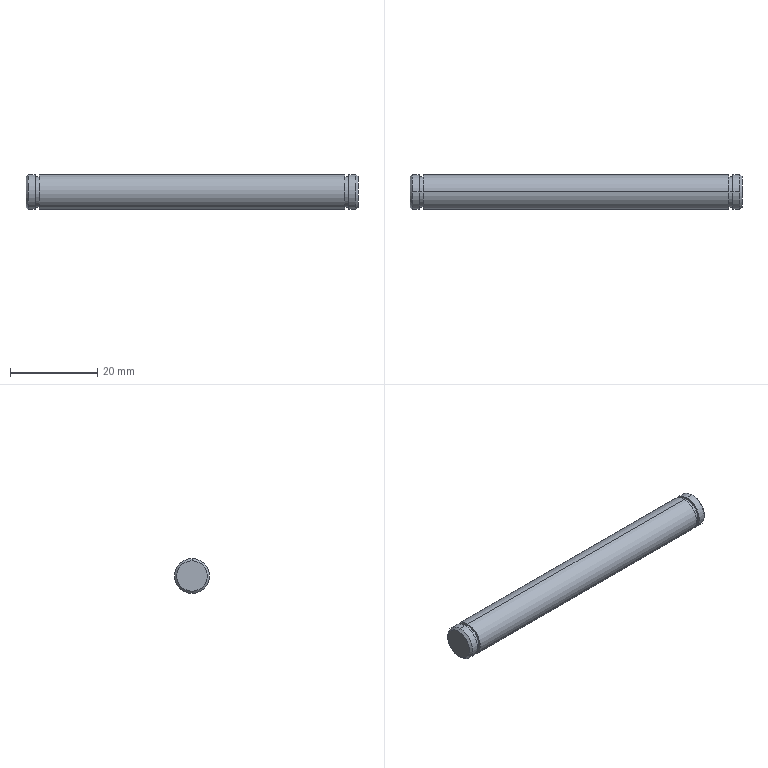Part | NX | features BREP 1 | 1 solid | 20 faces | box 76 x 8 x 8 mm | volume 3793 mm3 | cylinder 10 | plane 6 | cone 4 | commonest cylinder face diameters 8 x6 7 x4
STEP:
#1=CARTESIAN_POINT('',(76.,0.,3.5));
#2=VERTEX_POINT('',#1);
#3=CARTESIAN_POINT('',(76.,0.,-3.5));
#4=VERTEX_POINT('',#3);
#5=CARTESIAN_POINT('',(76.,0.,0.));
#6=DIRECTION('',(-1.,0.,0.));
#7=DIRECTION('',(0.,0.,1.));
#8=AXIS2_PLACEMENT_3D('',#5,#6,#7);
#9=CIRCLE('',#8,3.5);
#10=EDGE_CURVE('',#2,#4,#9,.T.);
#11=ORIENTED_EDGE('',*,*,#10,.T.);
#12=CARTESIAN_POINT('',(75.5,0.,-4.));
#13=VERTEX_POINT('',#12);
#14=CARTESIAN_POINT('',(76.,0.,-3.5));
#15=DIRECTION('',(-0.7071,0.,-0.7071));
#16=VECTOR('',#15,1000.);
#17=LINE('',#14,#16);
#18=EDGE_CURVE('',#13,#4,#17,.F.);
#19=ORIENTED_EDGE('',*,*,#18,.F.);
#20=CARTESIAN_POINT('',(75.5,0.,4.));
#21=VERTEX_POINT('',#20);
#22=CARTESIAN_POINT('',(75.5,0.,0.));
#23=DIRECTION('',(-1.,0.,0.));
#24=DIRECTION('',(0.,0.,1.));
#25=AXIS2_PLACEMENT_3D('',#22,#23,#24);
#26=CIRCLE('',#25,4.);
#27=EDGE_CURVE('',#21,#13,#26,.T.);
#28=ORIENTED_EDGE('',*,*,#27,.F.);
#29=CARTESIAN_POINT('',(76.,0.,3.5));
#30=DIRECTION('',(-0.7071,0.,0.7071));
#31=VECTOR('',#30,1000.);
#32=LINE('',#29,#31);
#33=EDGE_CURVE('',#21,#2,#32,.F.);
#34=ORIENTED_EDGE('',*,*,#33,.T.);
#35=EDGE_LOOP('',(#11,#19,#28,#34));
#36=FACE_BOUND('',#35,.T.);
#37=CARTESIAN_POINT('',(76.,0.,0.));
#38=DIRECTION('',(-1.,0.,0.));
#39=DIRECTION('',(0.,0.,1.));
#40=AXIS2_PLACEMENT_3D('',#37,#38,#39);
#41=CONICAL_SURFACE('',#40,3.5,0.7854);
#42=ADVANCED_FACE('',(#36),#41,.T.);
#43=ORIENTED_EDGE('',*,*,#27,.T.);
#44=CARTESIAN_POINT('',(73.9,0.,-4.));
#45=VERTEX_POINT('',#44);
#46=CARTESIAN_POINT('',(76.,0.,-4.));
#47=DIRECTION('',(-1.,0.,0.));
#48=VECTOR('',#47,1000.);
#49=LINE('',#46,#48);
#50=EDGE_CURVE('',#45,#13,#49,.F.);
#51=ORIENTED_EDGE('',*,*,#50,.F.);
#52=CARTESIAN_POINT('',(73.9,0.,4.));
#53=VERTEX_POINT('',#52);
#54=CARTESIAN_POINT('',(73.9,0.,0.));
#55=DIRECTION('',(-1.,0.,0.));
#56=DIRECTION('',(0.,0.,1.));
#57=AXIS2_PLACEMENT_3D('',#54,#55,#56);
#58=CIRCLE('',#57,4.);
#59=EDGE_CURVE('',#53,#45,#58,.T.);
#60=ORIENTED_EDGE('',*,*,#59,.F.);
#61=CARTESIAN_POINT('',(76.,0.,4.));
#62=DIRECTION('',(-1.,0.,0.));
#63=VECTOR('',#62,1000.);
#64=LINE('',#61,#63);
#65=EDGE_CURVE('',#53,#21,#64,.F.);
#66=ORIENTED_EDGE('',*,*,#65,.T.);
#67=EDGE_LOOP('',(#43,#51,#60,#66));
#68=FACE_BOUND('',#67,.T.);
#69=CARTESIAN_POINT('',(76.,0.,0.));
#70=DIRECTION('',(-1.,0.,0.));
#71=DIRECTION('',(0.,0.,1.));
#72=AXIS2_PLACEMENT_3D('',#69,#70,#71);
#73=CYLINDRICAL_SURFACE('',#72,4.);
#74=ADVANCED_FACE('',(#68),#73,.T.);
#75=CARTESIAN_POINT('',(73.9,0.,3.5));
#76=VERTEX_POINT('',#75);
#77=CARTESIAN_POINT('',(73.9,0.,-3.5));
#78=VERTEX_POINT('',#77);
#79=CARTESIAN_POINT('',(73.9,0.,0.));
#80=DIRECTION('',(-1.,0.,0.));
#81=DIRECTION('',(0.,0.,1.));
#82=AXIS2_PLACEMENT_3D('',#79,#80,#81);
#83=CIRCLE('',#82,3.5);
#84=EDGE_CURVE('',#76,#78,#83,.T.);
#85=ORIENTED_EDGE('',*,*,#84,.T.);
#86=CARTESIAN_POINT('',(73.,0.,-3.5));
#87=VERTEX_POINT('',#86);
#88=CARTESIAN_POINT('',(76.,0.,-3.5));
#89=DIRECTION('',(-1.,0.,0.));
#90=VECTOR('',#89,1000.);
#91=LINE('',#88,#90);
#92=EDGE_CURVE('',#87,#78,#91,.F.);
#93=ORIENTED_EDGE('',*,*,#92,.F.);
#94=CARTESIAN_POINT('',(73.,0.,3.5));
#95=VERTEX_POINT('',#94);
#96=CARTESIAN_POINT('',(73.,0.,0.));
#97=DIRECTION('',(-1.,0.,0.));
#98=DIRECTION('',(0.,0.,1.));
#99=AXIS2_PLACEMENT_3D('',#96,#97,#98);
#100=CIRCLE('',#99,3.5);
#101=EDGE_CURVE('',#95,#87,#100,.T.);
#102=ORIENTED_EDGE('',*,*,#101,.F.);
#103=CARTESIAN_POINT('',(76.,0.,3.5));
#104=DIRECTION('',(-1.,0.,0.));
#105=VECTOR('',#104,1000.);
#106=LINE('',#103,#105);
#107=EDGE_CURVE('',#95,#76,#106,.F.);
#108=ORIENTED_EDGE('',*,*,#107,.T.);
#109=EDGE_LOOP('',(#85,#93,#102,#108));
#110=FACE_BOUND('',#109,.T.);
#111=CARTESIAN_POINT('',(76.,0.,0.));
#112=DIRECTION('',(-1.,0.,0.));
#113=DIRECTION('',(0.,0.,1.));
#114=AXIS2_PLACEMENT_3D('',#111,#112,#113);
#115=CYLINDRICAL_SURFACE('',#114,3.5);
#116=ADVANCED_FACE('',(#110),#115,.T.);
#117=CARTESIAN_POINT('',(73.,0.,4.));
#118=VERTEX_POINT('',#117);
#119=CARTESIAN_POINT('',(73.,0.,-4.));
#120=VERTEX_POINT('',#119);
#121=CARTESIAN_POINT('',(73.,0.,0.));
#122=DIRECTION('',(-1.,0.,0.));
#123=DIRECTION('',(0.,0.,1.));
#124=AXIS2_PLACEMENT_3D('',#121,#122,#123);
#125=CIRCLE('',#124,4.);
#126=EDGE_CURVE('',#118,#120,#125,.T.);
#127=ORIENTED_EDGE('',*,*,#126,.T.);
#128=CARTESIAN_POINT('',(3.,0.,-4.));
#129=VERTEX_POINT('',#128);
#130=CARTESIAN_POINT('',(76.,0.,-4.));
#131=DIRECTION('',(-1.,0.,0.));
#132=VECTOR('',#131,1000.);
#133=LINE('',#130,#132);
#134=EDGE_CURVE('',#129,#120,#133,.F.);
#135=ORIENTED_EDGE('',*,*,#134,.F.);
#136=CARTESIAN_POINT('',(3.,0.,4.));
#137=VERTEX_POINT('',#136);
#138=CARTESIAN_POINT('',(3.,0.,0.));
#139=DIRECTION('',(-1.,0.,0.));
#140=DIRECTION('',(0.,0.,1.));
#141=AXIS2_PLACEMENT_3D('',#138,#139,#140);
#142=CIRCLE('',#141,4.);
#143=EDGE_CURVE('',#137,#129,#142,.T.);
#144=ORIENTED_EDGE('',*,*,#143,.F.);
#145=CARTESIAN_POINT('',(76.,0.,4.));
#146=DIRECTION('',(-1.,0.,0.));
#147=VECTOR('',#146,1000.);
#148=LINE('',#145,#147);
#149=EDGE_CURVE('',#137,#118,#148,.F.);
#150=ORIENTED_EDGE('',*,*,#149,.T.);
#151=EDGE_LOOP('',(#127,#135,#144,#150));
#152=FACE_BOUND('',#151,.T.);
#153=CARTESIAN_POINT('',(76.,0.,0.));
#154=DIRECTION('',(-1.,0.,0.));
#155=DIRECTION('',(0.,0.,1.));
#156=AXIS2_PLACEMENT_3D('',#153,#154,#155);
#157=CYLINDRICAL_SURFACE('',#156,4.);
#158=ADVANCED_FACE('',(#152),#157,.T.);
#159=CARTESIAN_POINT('',(3.,0.,3.5));
#160=VERTEX_POINT('',#159);
#161=CARTESIAN_POINT('',(3.,0.,-3.5));
#162=VERTEX_POINT('',#161);
#163=CARTESIAN_POINT('',(3.,0.,0.));
#164=DIRECTION('',(-1.,0.,0.));
#165=DIRECTION('',(0.,0.,1.));
#166=AXIS2_PLACEMENT_3D('',#163,#164,#165);
#167=CIRCLE('',#166,3.5);
#168=EDGE_CURVE('',#160,#162,#167,.T.);
#169=ORIENTED_EDGE('',*,*,#168,.T.);
#170=CARTESIAN_POINT('',(2.1,0.,-3.5));
#171=VERTEX_POINT('',#170);
#172=CARTESIAN_POINT('',(76.,0.,-3.5));
#173=DIRECTION('',(-1.,0.,0.));
#174=VECTOR('',#173,1000.);
#175=LINE('',#172,#174);
#176=EDGE_CURVE('',#171,#162,#175,.F.);
#177=ORIENTED_EDGE('',*,*,#176,.F.);
#178=CARTESIAN_POINT('',(2.1,0.,3.5));
#179=VERTEX_POINT('',#178);
#180=CARTESIAN_POINT('',(2.1,0.,0.));
#181=DIRECTION('',(-1.,0.,0.));
#182=DIRECTION('',(0.,0.,1.));
#183=AXIS2_PLACEMENT_3D('',#180,#181,#182);
#184=CIRCLE('',#183,3.5);
#185=EDGE_CURVE('',#179,#171,#184,.T.);
#186=ORIENTED_EDGE('',*,*,#185,.F.);
#187=CARTESIAN_POINT('',(76.,0.,3.5));
#188=DIRECTION('',(-1.,0.,0.));
#189=VECTOR('',#188,1000.);
#190=LINE('',#187,#189);
#191=EDGE_CURVE('',#179,#160,#190,.F.);
#192=ORIENTED_EDGE('',*,*,#191,.T.);
#193=EDGE_LOOP('',(#169,#177,#186,#192));
#194=FACE_BOUND('',#193,.T.);
#195=CARTESIAN_POINT('',(76.,0.,0.));
#196=DIRECTION('',(-1.,0.,0.));
#197=DIRECTION('',(0.,0.,1.));
#198=AXIS2_PLACEMENT_3D('',#195,#196,#197);
#199=CYLINDRICAL_SURFACE('',#198,3.5);
#200=ADVANCED_FACE('',(#194),#199,.T.);
#201=CARTESIAN_POINT('',(2.1,0.,4.));
#202=VERTEX_POINT('',#201);
#203=CARTESIAN_POINT('',(2.1,0.,-4.));
#204=VERTEX_POINT('',#203);
#205=CARTESIAN_POINT('',(2.1,0.,0.));
#206=DIRECTION('',(-1.,0.,0.));
#207=DIRECTION('',(0.,0.,1.));
#208=AXIS2_PLACEMENT_3D('',#205,#206,#207);
#209=CIRCLE('',#208,4.);
#210=EDGE_CURVE('',#202,#204,#209,.T.);
#211=ORIENTED_EDGE('',*,*,#210,.T.);
#212=CARTESIAN_POINT('',(0.5,0.,-4.));
#213=VERTEX_POINT('',#212);
#214=CARTESIAN_POINT('',(76.,0.,-4.));
#215=DIRECTION('',(-1.,0.,0.));
#216=VECTOR('',#215,1000.);
#217=LINE('',#214,#216);
#218=EDGE_CURVE('',#213,#204,#217,.F.);
#219=ORIENTED_EDGE('',*,*,#218,.F.);
#220=CARTESIAN_POINT('',(0.5,0.,4.));
#221=VERTEX_POINT('',#220);
#222=CARTESIAN_POINT('',(0.5,0.,0.));
#223=DIRECTION('',(-1.,0.,0.));
#224=DIRECTION('',(0.,0.,1.));
#225=AXIS2_PLACEMENT_3D('',#222,#223,#224);
#226=CIRCLE('',#225,4.);
#227=EDGE_CURVE('',#221,#213,#226,.T.);
#228=ORIENTED_EDGE('',*,*,#227,.F.);
#229=CARTESIAN_POINT('',(76.,0.,4.));
#230=DIRECTION('',(-1.,0.,0.));
#231=VECTOR('',#230,1000.);
#232=LINE('',#229,#231);
#233=EDGE_CURVE('',#221,#202,#232,.F.);
#234=ORIENTED_EDGE('',*,*,#233,.T.);
#235=EDGE_LOOP('',(#211,#219,#228,#234));
#236=FACE_BOUND('',#235,.T.);
#237=CARTESIAN_POINT('',(76.,0.,0.));
#238=DIRECTION('',(-1.,0.,0.));
#239=DIRECTION('',(0.,0.,1.));
#240=AXIS2_PLACEMENT_3D('',#237,#238,#239);
#241=CYLINDRICAL_SURFACE('',#240,4.);
#242=ADVANCED_FACE('',(#236),#241,.T.);
#243=CARTESIAN_POINT('',(0.,0.,3.5));
#244=VERTEX_POINT('',#243);
#245=CARTESIAN_POINT('',(0.,0.,-3.5));
#246=VERTEX_POINT('',#245);
#247=CARTESIAN_POINT('',(0.,0.,0.));
#248=DIRECTION('',(-1.,0.,0.));
#249=DIRECTION('',(0.,0.,1.));
#250=AXIS2_PLACEMENT_3D('',#247,#248,#249);
#251=CIRCLE('',#250,3.5);
#252=EDGE_CURVE('',#244,#246,#251,.T.);
#253=ORIENTED_EDGE('',*,*,#252,.F.);
#254=CARTESIAN_POINT('',(0.5,0.,4.));
#255=DIRECTION('',(0.7071,0.,0.7071));
#256=VECTOR('',#255,1000.);
#257=LINE('',#254,#256);
#258=EDGE_CURVE('',#244,#221,#257,.T.);
#259=ORIENTED_EDGE('',*,*,#258,.T.);
#260=ORIENTED_EDGE('',*,*,#227,.T.);
#261=CARTESIAN_POINT('',(0.5,0.,-4.));
#262=DIRECTION('',(0.7071,0.,-0.7071));
#263=VECTOR('',#262,1000.);
#264=LINE('',#261,#263);
#265=EDGE_CURVE('',#246,#213,#264,.T.);
#266=ORIENTED_EDGE('',*,*,#265,.F.);
#267=EDGE_LOOP('',(#253,#259,#260,#266));
#268=FACE_BOUND('',#267,.T.);
#269=CARTESIAN_POINT('',(0.5,0.,0.));
#270=DIRECTION('',(1.,0.,0.));
#271=DIRECTION('',(0.,0.,-1.));
#272=AXIS2_PLACEMENT_3D('',#269,#270,#271);
#273=CONICAL_SURFACE('',#272,4.,0.7854);
#274=ADVANCED_FACE('',(#268),#273,.T.);
#275=CARTESIAN_POINT('',(0.,0.,0.));
#276=DIRECTION('',(-1.,0.,0.));
#277=DIRECTION('',(0.,0.,1.));
#278=AXIS2_PLACEMENT_3D('',#275,#276,#277);
#279=CIRCLE('',#278,3.5);
#280=EDGE_CURVE('',#246,#244,#279,.T.);
#281=ORIENTED_EDGE('',*,*,#280,.T.);
#282=ORIENTED_EDGE('',*,*,#252,.T.);
#283=EDGE_LOOP('',(#281,#282));
#284=FACE_BOUND('',#283,.T.);
#285=CARTESIAN_POINT('',(0.,0.,0.));
#286=DIRECTION('',(1.,0.,0.));
#287=DIRECTION('',(0.,1.,0.));
#288=AXIS2_PLACEMENT_3D('',#285,#286,#287);
#289=PLANE('',#288);
#290=ADVANCED_FACE('',(#284),#289,.F.);
#291=ORIENTED_EDGE('',*,*,#258,.F.);
#292=ORIENTED_EDGE('',*,*,#280,.F.);
#293=ORIENTED_EDGE('',*,*,#265,.T.);
#294=CARTESIAN_POINT('',(0.5,0.,0.));
#295=DIRECTION('',(-1.,0.,0.));
#296=DIRECTION('',(0.,0.,1.));
#297=AXIS2_PLACEMENT_3D('',#294,#295,#296);
#298=CIRCLE('',#297,4.);
#299=EDGE_CURVE('',#213,#221,#298,.T.);
#300=ORIENTED_EDGE('',*,*,#299,.T.);
#301=EDGE_LOOP('',(#291,#292,#293,#300));
#302=FACE_BOUND('',#301,.T.);
#303=CARTESIAN_POINT('',(0.5,0.,0.));
#304=DIRECTION('',(1.,0.,0.));
#305=DIRECTION('',(0.,0.,-1.));
#306=AXIS2_PLACEMENT_3D('',#303,#304,#305);
#307=CONICAL_SURFACE('',#306,4.,0.7854);
#308=ADVANCED_FACE('',(#302),#307,.T.);
#309=ORIENTED_EDGE('',*,*,#218,.T.);
#310=CARTESIAN_POINT('',(2.1,0.,0.));
#311=DIRECTION('',(-1.,0.,0.));
#312=DIRECTION('',(0.,0.,1.));
#313=AXIS2_PLACEMENT_3D('',#310,#311,#312);
#314=CIRCLE('',#313,4.);
#315=EDGE_CURVE('',#204,#202,#314,.T.);
#316=ORIENTED_EDGE('',*,*,#315,.T.);
#317=ORIENTED_EDGE('',*,*,#233,.F.);
#318=ORIENTED_EDGE('',*,*,#299,.F.);
#319=EDGE_LOOP('',(#309,#316,#317,#318));
#320=FACE_BOUND('',#319,.T.);
#321=CARTESIAN_POINT('',(76.,0.,0.));
#322=DIRECTION('',(-1.,0.,0.));
#323=DIRECTION('',(0.,0.,1.));
#324=AXIS2_PLACEMENT_3D('',#321,#322,#323);
#325=CYLINDRICAL_SURFACE('',#324,4.);
#326=ADVANCED_FACE('',(#320),#325,.T.);
#327=ORIENTED_EDGE('',*,*,#210,.F.);
#328=ORIENTED_EDGE('',*,*,#315,.F.);
#329=EDGE_LOOP('',(#327,#328));
#330=FACE_BOUND('',#329,.T.);
#331=ORIENTED_EDGE('',*,*,#185,.T.);
#332=CARTESIAN_POINT('',(2.1,0.,0.));
#333=DIRECTION('',(-1.,0.,0.));
#334=DIRECTION('',(0.,0.,1.));
#335=AXIS2_PLACEMENT_3D('',#332,#333,#334);
#336=CIRCLE('',#335,3.5);
#337=EDGE_CURVE('',#171,#179,#336,.T.);
#338=ORIENTED_EDGE('',*,*,#337,.T.);
#339=EDGE_LOOP('',(#331,#338));
#340=FACE_BOUND('',#339,.T.);
#341=CARTESIAN_POINT('',(2.1,4.,0.));
#342=DIRECTION('',(-1.,0.,0.));
#343=DIRECTION('',(0.,0.,1.));
#344=AXIS2_PLACEMENT_3D('',#341,#342,#343);
#345=PLANE('',#344);
#346=ADVANCED_FACE('',(#330,#340),#345,.F.);
#347=ORIENTED_EDGE('',*,*,#176,.T.);
#348=CARTESIAN_POINT('',(3.,0.,0.));
#349=DIRECTION('',(-1.,0.,0.));
#350=DIRECTION('',(0.,0.,1.));
#351=AXIS2_PLACEMENT_3D('',#348,#349,#350);
#352=CIRCLE('',#351,3.5);
#353=EDGE_CURVE('',#162,#160,#352,.T.);
#354=ORIENTED_EDGE('',*,*,#353,.T.);
#355=ORIENTED_EDGE('',*,*,#191,.F.);
#356=ORIENTED_EDGE('',*,*,#337,.F.);
#357=EDGE_LOOP('',(#347,#354,#355,#356));
#358=FACE_BOUND('',#357,.T.);
#359=CARTESIAN_POINT('',(76.,0.,0.));
#360=DIRECTION('',(-1.,0.,0.));
#361=DIRECTION('',(0.,0.,1.));
#362=AXIS2_PLACEMENT_3D('',#359,#360,#361);
#363=CYLINDRICAL_SURFACE('',#362,3.5);
#364=ADVANCED_FACE('',(#358),#363,.T.);
#365=ORIENTED_EDGE('',*,*,#143,.T.);
#366=CARTESIAN_POINT('',(3.,0.,0.));
#367=DIRECTION('',(-1.,0.,0.));
#368=DIRECTION('',(0.,0.,1.));
#369=AXIS2_PLACEMENT_3D('',#366,#367,#368);
#370=CIRCLE('',#369,4.);
#371=EDGE_CURVE('',#129,#137,#370,.T.);
#372=ORIENTED_EDGE('',*,*,#371,.T.);
#373=EDGE_LOOP('',(#365,#372));
#374=FACE_BOUND('',#373,.T.);
#375=ORIENTED_EDGE('',*,*,#168,.F.);
#376=ORIENTED_EDGE('',*,*,#353,.F.);
#377=EDGE_LOOP('',(#375,#376));
#378=FACE_BOUND('',#377,.T.);
#379=CARTESIAN_POINT('',(3.,3.5,0.));
#380=DIRECTION('',(1.,0.,0.));
#381=DIRECTION('',(0.,1.,0.));
#382=AXIS2_PLACEMENT_3D('',#379,#380,#381);
#383=PLANE('',#382);
#384=ADVANCED_FACE('',(#374,#378),#383,.F.);
#385=ORIENTED_EDGE('',*,*,#134,.T.);
#386=CARTESIAN_POINT('',(73.,0.,0.));
#387=DIRECTION('',(-1.,0.,0.));
#388=DIRECTION('',(0.,0.,1.));
#389=AXIS2_PLACEMENT_3D('',#386,#387,#388);
#390=CIRCLE('',#389,4.);
#391=EDGE_CURVE('',#120,#118,#390,.T.);
#392=ORIENTED_EDGE('',*,*,#391,.T.);
#393=ORIENTED_EDGE('',*,*,#149,.F.);
#394=ORIENTED_EDGE('',*,*,#371,.F.);
#395=EDGE_LOOP('',(#385,#392,#393,#394));
#396=FACE_BOUND('',#395,.T.);
#397=CARTESIAN_POINT('',(76.,0.,0.));
#398=DIRECTION('',(-1.,0.,0.));
#399=DIRECTION('',(0.,0.,1.));
#400=AXIS2_PLACEMENT_3D('',#397,#398,#399);
#401=CYLINDRICAL_SURFACE('',#400,4.);
#402=ADVANCED_FACE('',(#396),#401,.T.);
#403=ORIENTED_EDGE('',*,*,#126,.F.);
#404=ORIENTED_EDGE('',*,*,#391,.F.);
#405=EDGE_LOOP('',(#403,#404));
#406=FACE_BOUND('',#405,.T.);
#407=ORIENTED_EDGE('',*,*,#101,.T.);
#408=CARTESIAN_POINT('',(73.,0.,0.));
#409=DIRECTION('',(-1.,0.,0.));
#410=DIRECTION('',(0.,0.,1.));
#411=AXIS2_PLACEMENT_3D('',#408,#409,#410);
#412=CIRCLE('',#411,3.5);
#413=EDGE_CURVE('',#87,#95,#412,.T.);
#414=ORIENTED_EDGE('',*,*,#413,.T.);
#415=EDGE_LOOP('',(#407,#414));
#416=FACE_BOUND('',#415,.T.);
#417=CARTESIAN_POINT('',(73.,4.,0.));
#418=DIRECTION('',(-1.,0.,0.));
#419=DIRECTION('',(0.,0.,1.));
#420=AXIS2_PLACEMENT_3D('',#417,#418,#419);
#421=PLANE('',#420);
#422=ADVANCED_FACE('',(#406,#416),#421,.F.);
#423=ORIENTED_EDGE('',*,*,#92,.T.);
#424=CARTESIAN_POINT('',(73.9,0.,0.));
#425=DIRECTION('',(-1.,0.,0.));
#426=DIRECTION('',(0.,0.,1.));
#427=AXIS2_PLACEMENT_3D('',#424,#425,#426);
#428=CIRCLE('',#427,3.5);
#429=EDGE_CURVE('',#78,#76,#428,.T.);
#430=ORIENTED_EDGE('',*,*,#429,.T.);
#431=ORIENTED_EDGE('',*,*,#107,.F.);
#432=ORIENTED_EDGE('',*,*,#413,.F.);
#433=EDGE_LOOP('',(#423,#430,#431,#432));
#434=FACE_BOUND('',#433,.T.);
#435=CARTESIAN_POINT('',(76.,0.,0.));
#436=DIRECTION('',(-1.,0.,0.));
#437=DIRECTION('',(0.,0.,1.));
#438=AXIS2_PLACEMENT_3D('',#435,#436,#437);
#439=CYLINDRICAL_SURFACE('',#438,3.5);
#440=ADVANCED_FACE('',(#434),#439,.T.);
#441=ORIENTED_EDGE('',*,*,#59,.T.);
#442=CARTESIAN_POINT('',(73.9,0.,0.));
#443=DIRECTION('',(-1.,0.,0.));
#444=DIRECTION('',(0.,0.,1.));
#445=AXIS2_PLACEMENT_3D('',#442,#443,#444);
#446=CIRCLE('',#445,4.);
#447=EDGE_CURVE('',#45,#53,#446,.T.);
#448=ORIENTED_EDGE('',*,*,#447,.T.);
#449=EDGE_LOOP('',(#441,#448));
#450=FACE_BOUND('',#449,.T.);
#451=ORIENTED_EDGE('',*,*,#84,.F.);
#452=ORIENTED_EDGE('',*,*,#429,.F.);
#453=EDGE_LOOP('',(#451,#452));
#454=FACE_BOUND('',#453,.T.);
#455=CARTESIAN_POINT('',(73.9,3.5,0.));
#456=DIRECTION('',(1.,0.,0.));
#457=DIRECTION('',(0.,1.,0.));
#458=AXIS2_PLACEMENT_3D('',#455,#456,#457);
#459=PLANE('',#458);
#460=ADVANCED_FACE('',(#450,#454),#459,.F.);
#461=ORIENTED_EDGE('',*,*,#50,.T.);
#462=CARTESIAN_POINT('',(75.5,0.,0.));
#463=DIRECTION('',(-1.,0.,0.));
#464=DIRECTION('',(0.,0.,1.));
#465=AXIS2_PLACEMENT_3D('',#462,#463,#464);
#466=CIRCLE('',#465,4.);
#467=EDGE_CURVE('',#13,#21,#466,.T.);
#468=ORIENTED_EDGE('',*,*,#467,.T.);
#469=ORIENTED_EDGE('',*,*,#65,.F.);
#470=ORIENTED_EDGE('',*,*,#447,.F.);
#471=EDGE_LOOP('',(#461,#468,#469,#470));
#472=FACE_BOUND('',#471,.T.);
#473=CARTESIAN_POINT('',(76.,0.,0.));
#474=DIRECTION('',(-1.,0.,0.));
#475=DIRECTION('',(0.,0.,1.));
#476=AXIS2_PLACEMENT_3D('',#473,#474,#475);
#477=CYLINDRICAL_SURFACE('',#476,4.);
#478=ADVANCED_FACE('',(#472),#477,.T.);
#479=ORIENTED_EDGE('',*,*,#18,.T.);
#480=CARTESIAN_POINT('',(76.,0.,0.));
#481=DIRECTION('',(-1.,0.,0.));
#482=DIRECTION('',(0.,0.,1.));
#483=AXIS2_PLACEMENT_3D('',#480,#481,#482);
#484=CIRCLE('',#483,3.5);
#485=EDGE_CURVE('',#4,#2,#484,.T.);
#486=ORIENTED_EDGE('',*,*,#485,.T.);
#487=ORIENTED_EDGE('',*,*,#33,.F.);
#488=ORIENTED_EDGE('',*,*,#467,.F.);
#489=EDGE_LOOP('',(#479,#486,#487,#488));
#490=FACE_BOUND('',#489,.T.);
#491=CARTESIAN_POINT('',(76.,0.,0.));
#492=DIRECTION('',(-1.,0.,0.));
#493=DIRECTION('',(0.,0.,1.));
#494=AXIS2_PLACEMENT_3D('',#491,#492,#493);
#495=CONICAL_SURFACE('',#494,3.5,0.7854);
#496=ADVANCED_FACE('',(#490),#495,.T.);
#497=ORIENTED_EDGE('',*,*,#10,.F.);
#498=ORIENTED_EDGE('',*,*,#485,.F.);
#499=EDGE_LOOP('',(#497,#498));
#500=FACE_BOUND('',#499,.T.);
#501=CARTESIAN_POINT('',(76.,3.5,0.));
#502=DIRECTION('',(-1.,0.,0.));
#503=DIRECTION('',(0.,0.,1.));
#504=AXIS2_PLACEMENT_3D('',#501,#502,#503);
#505=PLANE('',#504);
#506=ADVANCED_FACE('',(#500),#505,.F.);
#507=CLOSED_SHELL('',(#42,#74,#116,#158,#200,#242,#274,#290,#308,#326,#346,#364,#384,#402,#422,#440,#460,#478,#496,#506));
#508=MANIFOLD_SOLID_BREP('',#507);
#509=(LENGTH_UNIT()NAMED_UNIT(*)SI_UNIT(.MILLI.,.METRE.));
#510=UNCERTAINTY_MEASURE_WITH_UNIT(LENGTH_MEASURE(0.00001),#509,'','');
#511=(NAMED_UNIT(*)PLANE_ANGLE_UNIT()SI_UNIT($,.RADIAN.));
#512=(NAMED_UNIT(*)SI_UNIT($,.STERADIAN.)SOLID_ANGLE_UNIT());
#513=(GEOMETRIC_REPRESENTATION_CONTEXT(3)GLOBAL_UNCERTAINTY_ASSIGNED_CONTEXT((#510))GLOBAL_UNIT_ASSIGNED_CONTEXT((#509,#511,#512))REPRESENTATION_CONTEXT('',''));
#514=ADVANCED_BREP_SHAPE_REPRESENTATION('',(#508),#513);